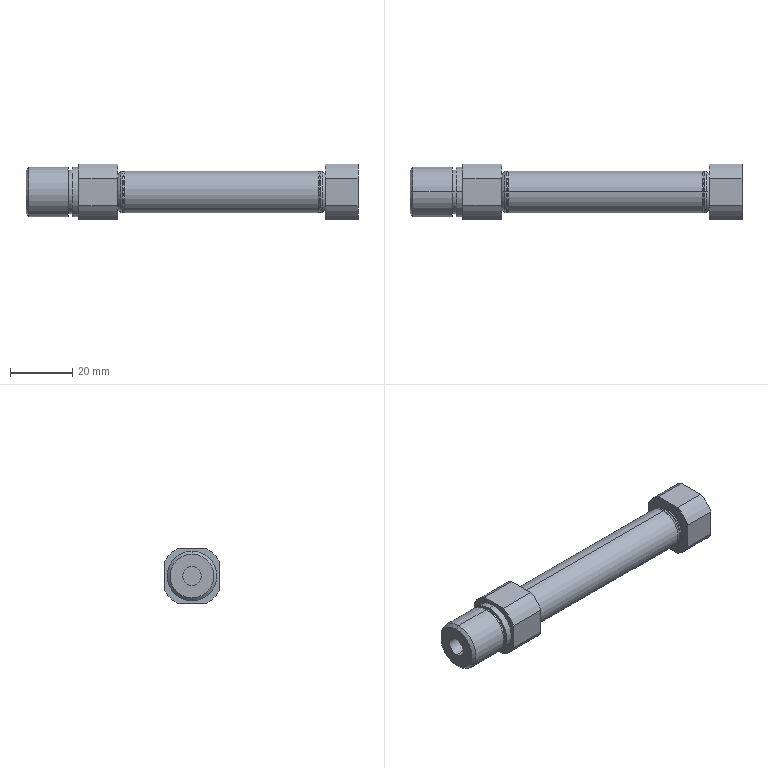Part | SolidWorks | features BaseBody 1 | 1 solid | 71 faces | box 107 x 18 x 18 mm | volume 12758 mm3 | cylinder 28 | plane 21 | cone 14 | spline 8 | commonest cylinder face diameters 20 x8 13.4 x6 4.134 x4 16 x4 6 x2 11.5 x2